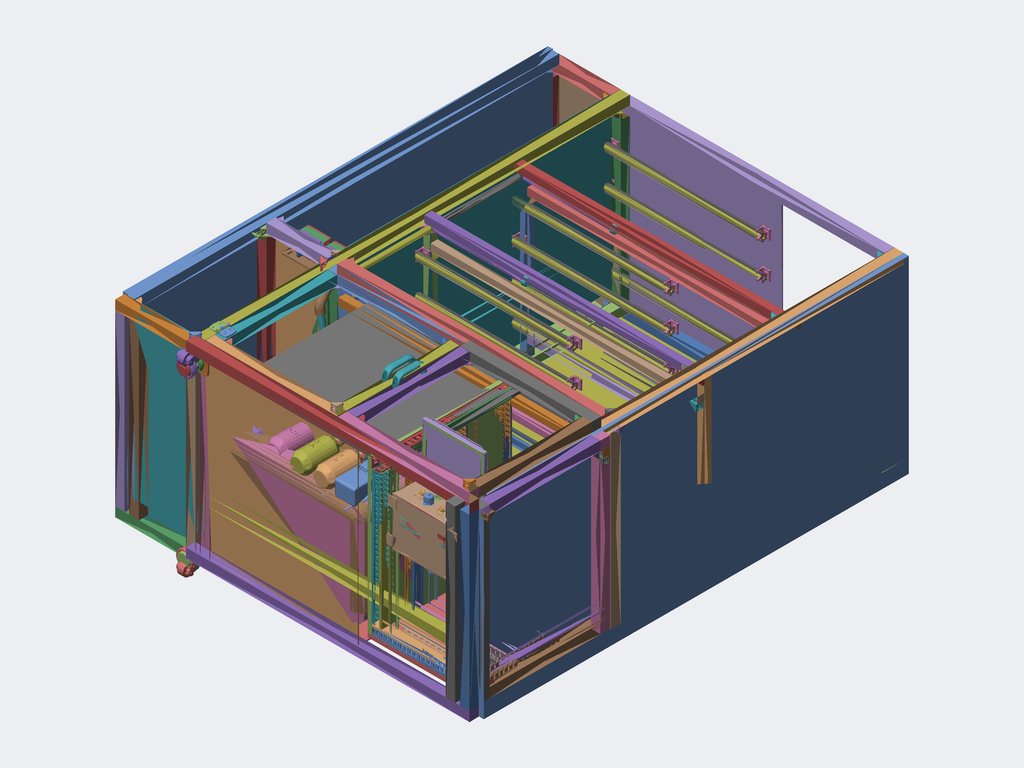Assembly | SolidWorks | 365 different items | 685 placed
Parts list (item | name | quantity | parent item | size | volume | features):
1 | (subassembly) | x1 | in 12 | 29 x 29.4 x 29.4 mm | 8063 mm3 | -
2 | (subassembly) | x1 | in 52 | 13.5 x 25.199 x 16.948 mm | 1807 mm3 | -
3 | (subassembly) | x1 | in 52 | 13.5 x 25.199 x 16.948 mm | 1807 mm3 | -
4 | (subassembly) | x1 | in 52 | 13.5 x 25.199 x 16.948 mm | 1807 mm3 | -
5 | (subassembly) | x1 | in 52 | 13.5 x 25.199 x 16.948 mm | 1807 mm3 | -
6 | (subassembly) | x1 | in 52 | - | - | -
7 | (subassembly) | x1 | in 52 | - | - | -
8 | (subassembly) | x1 | in 52 | - | - | -
9 | (subassembly) | x1 | in 52 | - | - | -
10 | (subassembly) | x1 | in 52 | - | - | -
11 | (subassembly) | x1 | in 52 | - | - | -
12 | (subassembly) | x1 | - | - | 806257 mm3 | -
13 | (subassembly) | x1 | in 50 | 13.5 x 25.199 x 16.948 mm | 1807 mm3 | -
14 | (subassembly) | x1 | in 124 | 23.449 x 13.5 x 13.5 mm | 1807 mm3 | -
15 | (subassembly) | x1 | in 53 | 13.5 x 26.207 x 19.88 mm | 1807 mm3 | -
16 | (subassembly) | x1 | in 53 | 13.5 x 26.207 x 19.88 mm | 1807 mm3 | -
17 | (subassembly) | x1 | in 53 | 13.5 x 26.207 x 19.88 mm | 1807 mm3 | -
18 | (subassembly) | x1 | in 53 | 13.5 x 26.207 x 19.88 mm | 1807 mm3 | -
19 | (subassembly) | x1 | in 53 | - | - | -
20 | (subassembly) | x1 | in 53 | - | - | -
21 | (subassembly) | x1 | in 53 | - | - | -
22 | (subassembly) | x1 | in 53 | - | - | -
23 | (subassembly) | x1 | in 80 | 664 x 385.75 x 394.5 mm | 131312 mm3 | -
24 | (subassembly) | x1 | in 53 | - | - | -
25 | (subassembly) | x1 | in 50 | - | - | -
26 | (subassembly) | x1 | in 53 | - | - | -
27 | (subassembly) | x1 | in 54 | 13.5 x 26.207 x 19.88 mm | 1807 mm3 | -
28 | (subassembly) | x1 | in 54 | 13.5 x 26.207 x 19.88 mm | 1807 mm3 | -
29 | (subassembly) | x1 | in 54 | 13.5 x 26.207 x 19.88 mm | 1807 mm3 | -
30 | (subassembly) | x1 | in 54 | 13.5 x 26.207 x 19.88 mm | 1807 mm3 | -
31 | (subassembly) | x1 | in 54 | - | - | -
32 | (subassembly) | x1 | in 54 | - | - | -
33 | (subassembly) | x1 | in 50 | - | - | -
34 | (subassembly) | x1 | - | 70 x 130 x 53 mm | 112751 mm3 | -
35 | (subassembly) | x1 | in 54 | - | - | -
36 | (subassembly) | x1 | in 55 | 13.5 x 26.207 x 19.88 mm | 1807 mm3 | -
37 | (subassembly) | x1 | in 55 | 13.5 x 26.207 x 19.88 mm | 1807 mm3 | -
38 | (subassembly) | x1 | in 55 | 13.5 x 26.207 x 19.88 mm | 1807 mm3 | -
39 | (subassembly) | x1 | in 55 | 13.5 x 26.207 x 19.88 mm | 1807 mm3 | -
40 | (subassembly) | x1 | in 55 | - | - | -
41 | (subassembly) | x1 | in 55 | - | - | -
42 | (subassembly) | x1 | in 55 | - | - | -
43 | (subassembly) | x1 | in 55 | - | - | -
44 | (subassembly) | x1 | in 55 | - | - | -
45 | (subassembly) | x1 | - | 77 x 48 x 16 mm | 26381 mm3 | -
46 | (subassembly) | x1 | in 50 | - | - | -
47 | (subassembly) | x1 | in 50 | - | - | -
48 | (subassembly) | x1 | in 50 | - | - | -
49 | (subassembly) | x1 | in 50 | - | - | -
50 | (subassembly) | x1 | in 126 | 346.5 x 25.199 x 16.948 mm | 7226 mm3 | -
51 | (subassembly) | x1 | in 127 | 346.5 x 25.199 x 16.948 mm | 7226 mm3 | -
52 | (subassembly) | x1 | in 129 | 346.5 x 25.199 x 16.948 mm | 7226 mm3 | -
53 | (subassembly) | x1 | in 113 | 346.5 x 26.207 x 19.88 mm | 7226 mm3 | -
54 | (subassembly) | x1 | in 114 | 346.5 x 26.207 x 19.88 mm | 7226 mm3 | -
55 | (subassembly) | x1 | in 115 | 346.5 x 26.207 x 19.88 mm | 7226 mm3 | -
56 | (subassembly) | x1 | in 45 | - | - | -
57 | (subassembly) | x1 | in 76 | 408 x 327.5 x 71.18 mm | 128215 mm3 | -
58 | (subassembly) | x1 | in 59 | 610 x 320 x 430 mm | 61319662 mm3 | -
59 | (subassembly) | x1 | - | - | - | -
60 | (subassembly) | x5 | in 97 | 23.094 x 55.999 x 32.35 mm | 8057 mm3 | -
61 | (subassembly) | x1 | in 98 | 23.094 x 55.999 x 32.35 mm | 8057 mm3 | -
62 | (subassembly) | x1 | in 99 | 23.094 x 55.999 x 32.35 mm | 8057 mm3 | -
63 | (subassembly) | x1 | in 137 | 41.648 x 27.781 x 48.022 mm | 12703 mm3 | -
64 | (subassembly) | x1 | in 137 | - | - | -
65 | (subassembly) | x1 | in 116 | 38.308 x 50.8 x 53.348 mm | 36744 mm3 | -
66 | (subassembly) | x5 | in 91 | 660 x 66.14 x 97.82 mm | 1407720 mm3 | -
67 | (subassembly) | x2 | in 45 | - | - | -
68 | (subassembly) | x1 | in 92 | 660 x 66.14 x 97.82 mm | 1407720 mm3 | -
69 | (subassembly) | x1 | in 93 | 660 x 66.14 x 97.82 mm | 1407720 mm3 | -
70 | (subassembly) | x1 | in 77 | 56.3 x 65.53 x 50.125 mm | 38385 mm3 | -
71 | (subassembly) | x1 | in 77 | 56.3 x 65.53 x 50.125 mm | 38385 mm3 | -
72 | (subassembly) | x1 | in 77 | 56.3 x 65.53 x 50.125 mm | 38385 mm3 | -
73 | (subassembly) | x1 | in 119 | - | - | -
74 | (subassembly) | x1 | in 77 | 56.3 x 65.53 x 50.125 mm | 38385 mm3 | -
75 | (subassembly) | x1 | in 77 | 56.3 x 65.53 x 50.125 mm | 38385 mm3 | -
76 | (subassembly) | x1 | in 59 | - | 1784290 mm3 | -
77 | (subassembly) | x1 | in 76 | - | 191920 mm3 | -
78 | (subassembly) | x1 | in 116 | 44.298 x 85.549 x 87.319 mm | 55176 mm3 | -
79 | (subassembly) | x1 | in 120 | 6.25 x 60 x 64.152 mm | 14252 mm3 | -
80 | (subassembly) | x1 | - | - | - | -
81 | (subassembly) | x1 | in 59 | 27.5 x 27.5 x 265.5 mm | 30904 mm3 | -
82 | (subassembly) | x1 | in 88 | - | - | -
83 | (subassembly) | x1 | in 88 | - | - | -
84 | (subassembly) | x3 | in 95, 106, 117 | 32.512 x 58.766 x 128.692 mm | 33883 mm3 | -
85 | (subassembly) | x1 | in 88 | 101 x 80 x 82.8 mm | 248675 mm3 | -
86 | (subassembly) | x1 | in 88 | - | - | -
87 | (subassembly) | x1 | in 88 | 101 x 80 x 82.8 mm | 248693 mm3 | -
88 | (subassembly) | x1 | - | 80 x 82.8 x 822 mm | 497420 mm3 | -
89 | (subassembly) | x1 | - | 676.368 x 834.5 x 490.186 mm | 2486985 mm3 | -
90 | (subassembly) | x3 | in 89 | 676.368 x 34.5 x 490.186 mm | 828995 mm3 | -
91 | (subassembly) | x5 | in 97 | 664 x 107.82 x 71.14 mm | 1474678 mm3 | -
92 | (subassembly) | x1 | in 98 | 664 x 107.82 x 71.14 mm | 1474678 mm3 | -
93 | (subassembly) | x1 | in 99 | 664 x 107.82 x 71.14 mm | 1474678 mm3 | -
94 | (subassembly) | x1 | - | - | 7857189 mm3 | -
95 | (subassembly) | x1 | in 126 | 174.317 x 60.383 x 32.544 mm | 89512 mm3 | -
96 | (subassembly) | x1 | in 94 | - | 7857189 mm3 | -
97 | (subassembly) | x5 | in 96, 100 | 107.82 x 101.739 x 678.552 mm | 1521216 mm3 | -
98 | (subassembly) | x1 | in 100 | 107.82 x 101.739 x 678.552 mm | 1521216 mm3 | -
99 | (subassembly) | x1 | in 100 | 107.82 x 101.739 x 678.552 mm | 1521216 mm3 | -
100 | (subassembly) | x1 | in 96 | - | 4563696 mm3 | -
101 | (subassembly) | x5 | in 97 | 17.4 x 36.23 x 48.652 mm | 7597 mm3 | -
102 | (subassembly) | x1 | in 98 | 17.4 x 36.23 x 48.652 mm | 7597 mm3 | -
103 | (subassembly) | x1 | in 99 | 17.4 x 36.23 x 48.652 mm | 7597 mm3 | -
104 | (subassembly) | x1 | in 125 | - | 2028858 mm3 | -
105 | (subassembly) | x1 | - | 1112 x 1800 x 795 mm | 20539975 mm3 | -
106 | (subassembly) | x1 | in 127 | 174.317 x 60.383 x 32.544 mm | 89512 mm3 | -
107 | (subassembly) | x1 | in 137 | 56.5 x 114.123 x 126.119 mm | 204524 mm3 | -
108 | (subassembly) | x1 | in 137 | 162.238 x 114.123 x 56.5 mm | 232338 mm3 | -
109 | (subassembly) | x5 | in 97 | 48.245 x 49.817 x 548.245 mm | 30830 mm3 | -
110 | (subassembly) | x1 | in 98 | 48.245 x 49.817 x 548.245 mm | 30830 mm3 | -
111 | (subassembly) | x1 | in 99 | 48.245 x 49.817 x 548.245 mm | 30830 mm3 | -
112 | (subassembly) | x1 | in 76 | - | 1269065 mm3 | -
113 | (subassembly) | x1 | in 116 | 422.844 x 53.25 x 32.766 mm | 119416 mm3 | -
114 | (subassembly) | x1 | in 116 | 426.966 x 53.25 x 32.766 mm | 119416 mm3 | -
115 | (subassembly) | x1 | in 116 | 422.797 x 53.25 x 32.766 mm | 119416 mm3 | -
116 | (subassembly) | x1 | in 125 | 428.236 x 959.541 x 415.929 mm | 725638 mm3 | -
117 | (subassembly) | x1 | in 129 | 174.317 x 60.383 x 32.544 mm | 89512 mm3 | -
118 | (subassembly) | x1 | in 120 | - | 494108 mm3 | -
119 | (subassembly) | x1 | - | - | - | -
120 | (subassembly) | x1 | in 73 | - | - | -
121 | (subassembly) | x1 | in 73 | 292.1 x 154.813 x 421.143 mm | 614239 mm3 | -
122 | (subassembly) | x1 | in 126 | 388.057 x 91.084 x 21.234 mm | 100985 mm3 | -
123 | (subassembly) | x2 | in 127, 129 | 388.057 x 91.084 x 21.234 mm | 100985 mm3 | -
124 | (subassembly) | x1 | in 104 | 38.38 x 1164 x 21.234 mm | 226503 mm3 | -
125 | (subassembly) | x1 | - | - | 2759072 mm3 | -
126 | (subassembly) | x1 | in 104 | 415.26 x 140.383 x 32.766 mm | 299661 mm3 | -
127 | (subassembly) | x1 | in 104 | 415.26 x 140.383 x 32.766 mm | 299661 mm3 | -
128 | (subassembly) | x1 | in 105 | 982 x 1800 x 795 mm | 20539975 mm3 | -
129 | (subassembly) | x1 | in 104 | 432.043 x 140.383 x 32.766 mm | 310066 mm3 | -
130 | (subassembly) | x5 | in 101 | 17.4 x 34.9 x 11.547 mm | 2470 mm3 | -
131 | (subassembly) | x1 | in 102 | 17.4 x 34.9 x 11.547 mm | 2470 mm3 | -
132 | (subassembly) | x1 | in 103 | 17.4 x 34.9 x 11.547 mm | 2470 mm3 | -
133 | (subassembly) | x1 | in 135 | 14 x 137.38 x 15.856 mm | 6154 mm3 | -
134 | (subassembly) | x1 | in 135 | 156 x 156 x 86 mm | 282738 mm3 | -
135 | (subassembly) | x1 | in 59 | 156 x 335.859 x 98.479 mm | 1667612 mm3 | -
136 | (subassembly) | x1 | in 108 | 79 x 109.5 x 56.5 mm | 176709 mm3 | -
137 | (subassembly) | x1 | in 104 | 415.889 x 172.793 x 383.815 mm | 846980 mm3 | features CompositeCurve 4
138 | (subassembly) | x1 | in 59 | 134.4 x 256.29 x 184.2 mm | 2229611 mm3 | -
139 | (subassembly) | x1 | in 12 | 29 x 29.4 x 29.4 mm | 8063 mm3 | -
140 | (subassembly) | x1 | in 137 | 69.85 x 87.046 x 27.178 mm | 35204 mm3 | -
141 | (subassembly) | x1 | in 137 | - | - | -
142 | (subassembly) | x1 | in 137 | 69.85 x 87.046 x 27.178 mm | 35204 mm3 | -
143 | (subassembly) | x1 | in 140 | 22.25 x 60.757 x 25.693 mm | 8431 mm3 | -
144 | (subassembly) | x1 | in 142 | 22.25 x 60.757 x 25.693 mm | 8431 mm3 | -
145 | (subassembly) | x1 | in 116 | 25.302 x 60.757 x 24.143 mm | 8431 mm3 | -
146 | (subassembly) | x1 | in 80 | - | - | -
147 | (subassembly) | x1 | in 50 | 13.5 x 25.199 x 16.948 mm | 1807 mm3 | -
148 | (subassembly) | x1 | in 50 | 13.5 x 25.199 x 16.948 mm | 1807 mm3 | -
149 | (subassembly) | x1 | in 51 | 13.5 x 25.199 x 16.948 mm | 1807 mm3 | -
150 | (subassembly) | x10 | in 12 | 29 x 29.4 x 29.4 mm | 8063 mm3 | -
151 | (subassembly) | x1 | in 51 | 13.5 x 25.199 x 16.948 mm | 1807 mm3 | -
152 | (subassembly) | x1 | in 51 | 13.5 x 25.199 x 16.948 mm | 1807 mm3 | -
153 | (subassembly) | x1 | in 51 | 13.5 x 25.199 x 16.948 mm | 1807 mm3 | -
154 | (subassembly) | x1 | in 51 | - | - | -
155 | (subassembly) | x1 | in 51 | - | - | -
156 | (subassembly) | x1 | in 51 | - | - | -
157 | (subassembly) | x1 | in 51 | - | - | -
158 | (subassembly) | x1 | in 51 | - | - | -
159 | (subassembly) | x1 | in 51 | - | - | -
160 | (subassembly) | x1 | in 50 | 13.5 x 25.199 x 16.948 mm | 1807 mm3 | -
161 | - | x1 | in 120 | 7.5 x 222.25 x 35 mm | 9598 mm3 | features BaseBody 1
162 | - | x1 | in 12 | 29 x 29.4 x 29.4 mm | 8063 mm3 | features BaseBody 1
163 | - | x1 | in 12 | 29 x 29.4 x 29.4 mm | 8063 mm3 | features BaseBody 1
164 | - | x1 | in 12 | 29 x 29.4 x 29.4 mm | 8063 mm3 | features BaseBody 1
165 | - | x1 | in 12 | 29 x 29.4 x 29.4 mm | 8063 mm3 | features BaseBody 1
166 | - | x1 | in 12 | 29 x 29.4 x 29.4 mm | 8063 mm3 | features BaseBody 1
167 | - | x1 | in 12 | 29 x 29.4 x 29.4 mm | 8063 mm3 | features BaseBody 1
168 | - | x1 | in 12 | 29 x 29.4 x 29.4 mm | 8063 mm3 | features BaseBody 1
169 | - | x1 | in 12 | 29 x 29.4 x 29.4 mm | 8063 mm3 | features BaseBody 1
170 | - | x1 | in 12 | 29 x 29.4 x 29.4 mm | 8063 mm3 | features BaseBody 1
171 | - | x1 | in 12 | 29 x 29.4 x 29.4 mm | 8063 mm3 | features BaseBody 1
172 | - | x4 | in 137, 143, 144, 145 | 22.25 x 25.693 x 60.757 mm | 8431 mm3 | features BaseBody 1
173 | - | x1 | in 12 | 29 x 29.4 x 29.4 mm | 8063 mm3 | features BaseBody 1
174 | - | x1 | in 12 | 29 x 29.4 x 29.4 mm | 8063 mm3 | features BaseBody 1
175 | - | x1 | in 12 | 29 x 29.4 x 29.4 mm | 8063 mm3 | features BaseBody 1
176 | - | x1 | in 12 | 29 x 29.4 x 29.4 mm | 8063 mm3 | features BaseBody 1
177 | - | x1 | in 12 | 29 x 29.4 x 29.4 mm | 8063 mm3 | features BaseBody 1
178 | - | x1 | in 12 | 29 x 29.4 x 29.4 mm | 8063 mm3 | features BaseBody 1
179 | - | x1 | in 12 | 29 x 29.4 x 29.4 mm | 8063 mm3 | features BaseBody 1
180 | - | x1 | in 12 | 29 x 29.4 x 29.4 mm | 8063 mm3 | features BaseBody 1
181 | - | x1 | in 12 | 29 x 29.4 x 29.4 mm | 8063 mm3 | features BaseBody 1
182 | - | x12 | in 1, 139, 150 | 29 x 29.4 x 29.4 mm | 8063 mm3 | features BaseBody 1
183 | - | x1 | in 112 | 85.56 x 83.56 x 203.378 mm | 49544 mm3 | features BaseBody 2
184 | - | x1 | in 135 | 67.479 x 24 x 282.859 mm | 49181 mm3 | features BaseBody 4
185 | - | x8 | in 104, 113, 114, 115, 126, 127, 129, 137 | 49.53 x 49.53 x 29.465 mm | 26737 mm3 | features BaseBody 1
186 | - | x1 | in 85 | 101 x 80 x 82.8 mm | 248675 mm3 | features BaseBody 9
187 | - | x1 | in 87 | 101 x 80 x 82.8 mm | 248693 mm3 | features BaseBody 9
188 | - | x12 | in 90 | 670 x 24 x 40.186 mm | 190097 mm3 | features BaseBody 2, ICE 1
189 | - | x1 | in 121 | 206.936 x 292.1 x 154.813 mm | 362955 mm3 | features BaseBody 1
190 | - | x1 | in 45 | 77 x 48 x 16 mm | 26381 mm3 | features BaseBody 3
191 | - | x1 | in 138 | 134.4 x 184.2 x 103.29 mm | 334800 mm3 | features BaseBody 3
192 | - | x7 | in 101, 102, 103 | - | 2700 mm3 | features BaseBody 1
193 | - | x2 | in 79, 120 | 64.028 x 5 x 60 mm | 11357 mm3 | features BaseBody 1
194 | - | x5 | in 70, 71, 72, 74, 75 | 65.53 x 40.25 x 56.3 mm | 27428 mm3 | features BaseBody 3
195 | - | x1 | in 79 | 63.246 x 1.25 x 48.204 mm | 2895 mm3 | features BaseBody 1
196 | - | x1 | in 120 | 43.7 x 5.75 x 42 mm | 7228 mm3 | features BaseBody 1
197 | - | x2 | - | 800 x 1800 x 20 mm | 28800000 mm3 | features Extrusion 1
198 | - | x1 | in 81 | 18.244 x 265.5 x 15.8 mm | 6663 mm3 | features BaseBody 1
199 | - | x1 | in 138 | 134.4 x 134.4 x 157.5 mm | 1797413 mm3 | features BaseBody 2
200 | - | x11 | in 95, 106, 107, 108, 117, 137 | 61.119 x 35.745 x 32.544 mm | 27815 mm3 | features BaseBody 2
201 | - | x1 | in 112 | 85.56 x 83.56 x 203.378 mm | 49595 mm3 | features BaseBody 2
202 | - | x1 | in 112 | 85.56 x 83.56 x 203.378 mm | 49646 mm3 | features BaseBody 2
203 | - | x1 | in 81 | - | - | features RefSurface 1
204 | - | x7 | in 60, 61, 62 | 23.094 x 24.5 x 20 mm | 3796 mm3 | features BaseBody 2
205 | - | x5 | in 70, 71, 72, 74, 75 | 19.6 x 11.9 x 19.6 mm | 729.046 mm3 | features BaseBody 1
206 | - | x1 | in 76 | 525 x 80 x 5 mm | 194805 mm3 | features BaseBody 11
207 | - | x1 | in 80 | 666 x 555 x 451 mm | 9776880 mm3 | features BaseBody 2
208 | - | x2 | in 73 | 50.41 x 34 x 34 mm | 20764 mm3 | features BaseBody 1
209 | - | x1 | in 73 | 26 x 30.7 x 31 mm | 6883 mm3 | features BaseBody 1
210 | - | x1 | in 124 | 21.234 x 384.346 x 21.234 mm | 76950 mm3 | features BaseBody 1
211 | - | x1 | in 124 | 21.234 x 384.6 x 21.234 mm | 78104 mm3 | features BaseBody 1
212 | - | x1 | in 124 | 21.234 x 344.346 x 21.234 mm | 69645 mm3 | features BaseBody 1
213 | - | x3 | in 113, 114, 115 | 381 x 21.235 x 21.234 mm | 75088 mm3 | features BaseBody 1, ICE 1
214 | - | x1 | in 116 | 86.694 x 862.008 x 383.174 mm | 199579 mm3 | features BaseBody 3
215 | - | x1 | in 133 | 14 x 15.856 x 22.23 mm | 2429 mm3 | features BaseBody 2
216 | - | x5 | in 70, 71, 72, 74, 75 | 39.14 x 10.37 x 38.9 mm | 2813 mm3 | features BaseBody 1
217 | - | x1 | in 133 | 14 x 15.856 x 22.23 mm | 1913 mm3 | features BaseBody 2
218 | - | x7 | in 101, 102, 103 | 14 x 15.856 x 22.23 mm | 2429 mm3 | features BaseBody 2
219 | - | x1 | - | 1190 x 1150 x 790 mm | 14724000 mm3 | features BaseBody 16
220 | - | x1 | - | 1500 x 1840 x 800 mm | 56736000 mm3 | features BaseBody 43
221 | - | x1 | in 138 | - | - | features BaseBody 2, RefSurface 1
222 | - | x1 | in 134 | 3 x 15 x 60 mm | 2677 mm3 | features BaseBody 1
223 | - | x1 | in 136 | 79 x 56.5 x 109.5 mm | 176709 mm3 | features BaseBody 10
224 | - | x2 | in 107, 137 | 79 x 56.5 x 109.5 mm | 176709 mm3 | features BaseBody 10
225 | - | x9 | in 116, 126, 127, 129, 137 | 70.104 x 49.555 x 29.007 mm | 32399 mm3 | features BaseBody 1
226 | - | x49 | in 109, 110, 111 | 48.245 x 48.245 x 49.817 mm | 4404 mm3 | features BaseBody 1
227 | - | x5 | in 70, 71, 72, 74, 75 | 31.23 x 17.45 x 36.34 mm | 4500 mm3 | features BaseBody 1
228 | - | x1 | - | 1160 x 720 x 3 mm | 2505600 mm3 | features Extrusion 1
229 | - | x1 | - | 720 x 260 x 5 mm | 936000 mm3 | features Extrusion 1
230 | - | x1 | in 146 | 40 x 40.1 x 555 mm | 152024 mm3 | features BaseBody 2
231 | - | x1 | in 146 | 40 x 40.1 x 555 mm | 152024 mm3 | features BaseBody 2
232 | - | x1 | in 146 | 40 x 40.1 x 395 mm | 108160 mm3 | features BaseBody 2
233 | - | x3 | in 146 | 40 x 40.1 x 395 mm | 108160 mm3 | features BaseBody 2
234 | - | x1 | in 146 | 40 x 40.1 x 570 mm | 156325 mm3 | features BaseBody 2
235 | - | x3 | in 146 | 40 x 40.1 x 570 mm | 156325 mm3 | features BaseBody 2
236 | - | x1 | in 58 | 608 x 220 x 428 mm | 56795852 mm3 | features BaseBody 1
237 | - | x1 | in 135 | 144 x 115 x 74 mm | 1223728 mm3 | features BaseBody 1
238 | - | x10 | in 70, 71, 72, 74, 75 | 7.18 x 1.7 x 7.64 mm | 58.331 mm3 | features BaseBody 1
239 | - | x1 | in 112 | 85 x 70 x 206 mm | 1070549 mm3 | features BaseBody 2
240 | - | x1 | in 96 | 355 x 5 x 135 mm | 128920 mm3 | features BaseBody 1, ICE 1
241 | - | x1 | in 134 | 150 x 153 x 80 mm | 237530 mm3 | features BaseBody 1
242 | - | x1 | in 23 | 7.5 x 35 x 637 mm | 27495 mm3 | features BaseBody 1
243 | - | x1 | in 23 | 7.5 x 35 x 386 mm | 16663 mm3 | features BaseBody 1
244 | - | x1 | in 23 | 7.5 x 35 x 386 mm | 16663 mm3 | features BaseBody 1
245 | - | x1 | in 23 | 7.5 x 35 x 386 mm | 16663 mm3 | features BaseBody 1
246 | - | x1 | in 23 | 7.5 x 35 x 637 mm | 27495 mm3 | features BaseBody 1
247 | - | x1 | in 23 | 7.5 x 35 x 610 mm | 26333 mm3 | features BaseBody 1
248 | - | x4 | in 81 | 16.932 x 14.78 x 0.889 mm | 89.694 mm3 | features BaseBody 1
249 | - | x15 | in 70, 71, 72, 74, 75 | 10.75 x 13.9 x 10.75 mm | 660.288 mm3 | features BaseBody 1
250 | - | x2 | in 81 | - | - | features RefSurface 1
251 | - | x2 | in 96 | 577 x 5 x 105 mm | 122030 mm3 | features BaseBody 1, ICE 1
252 | - | x1 | in 81 | 16 x 18.475 x 5 mm | 804.205 mm3 | features BaseBody 1
253 | - | x1 | in 134 | 156 x 8 x 86 mm | 42531 mm3 | features BaseBody 2
254 | - | x24 | in 90 | 40 x 32.5 x 32.5 mm | 8576 mm3 | features BaseBody 1
255 | - | x3 | in 122, 123 | 67 x 21.234 x 21.234 mm | 13325 mm3 | features BaseBody 1, ICE 1
256 | - | x1 | in 135 | 31.058 x 31.058 x 249.412 mm | 105798 mm3 | features BaseBody 5
257 | - | x9 | in 104, 113, 114, 115, 126, 127, 129 | 20.956 x 32.766 x 32.766 mm | 10405 mm3 | features BaseBody 1
258 | - | x7 | in 130, 131, 132 | 17.4 x 34.9 x 11.547 mm | 2470 mm3 | features BaseBody 4
259 | - | x3 | in 122, 123 | 290 x 21.234 x 21.234 mm | 58049 mm3 | features BaseBody 1
260 | - | x5 | in 70, 71, 72, 74, 75 | 21 x 4 x 40.5 mm | 817.162 mm3 | features BaseBody 1
261 | - | x7 | in 91, 92, 93 | 664 x 107.82 x 40 mm | 66958 mm3 | features BaseBody 2
262 | - | x7 | in 66, 68, 69 | 660 x 60.3 x 97.82 mm | 1057763 mm3 | features BaseBody 1
263 | - | x25 | in 2, 3, 4, 5, 13, 14, 15, 16, 17, 18, 27, 28, 29, 30, 36, 37, 38, 39, 147, 148, 149, 151, 152, 153, 160 | 13.5 x 13.5 x 23.449 mm | 1807 mm3 | features BaseBody 1
264 | - | x7 | in 66, 68, 69 | 660 x 11.68 x 97.82 mm | 349958 mm3 | features BaseBody 1
265 | - | x1 | in 133 | 6.9 x 97.77 x 6.9 mm | 1812 mm3 | features BaseBody 1
266 | - | x3 | in 122, 123 | 145.797 x 21.234 x 21.234 mm | 29608 mm3 | features BaseBody 1
267 | - | x1 | in 128 | 260 x 560 x 5 mm | 728000 mm3 | features BaseBody 1
268 | - | x1 | in 128 | 260 x 5 x 720 mm | 936000 mm3 | features BaseBody 1
269 | - | x1 | in 128 | 645 x 555 x 10 mm | 3579750 mm3 | features BaseBody 1, ICE 1
270 | - | x1 | in 128 | 647 x 1160 x 5 mm | 3752600 mm3 | features BaseBody 1, ICE 1
271 | - | x1 | in 120 | 25.3 x 89.537 x 86.5 mm | 117361 mm3 | features BaseBody 1
272 | - | x2 | in 34 | 130 x 53 x 26 mm | 56376 mm3 | features BaseBody 1
273 | - | x1 | in 128 | 330 x 5 x 790 mm | 1246600 mm3 | features BaseBody 1
274 | - | x1 | in 128 | 647 x 5 x 755 mm | 2438375 mm3 | features BaseBody 1, ICE 1
275 | - | x1 | in 128 | 647 x 5 x 685 mm | 2209850 mm3 | features BaseBody 1, ICE 1
276 | - | x1 | in 128 | 260 x 1160 x 5 mm | 1508000 mm3 | features BaseBody 1
277 | - | x1 | in 128 | 647 x 560 x 5 mm | 1811600 mm3 | features BaseBody 1, ICE 1
278 | - | x1 | in 128 | 647 x 5 x 720 mm | 2329200 mm3 | features BaseBody 1, ICE 1
279 | - | x7 | in 60, 61, 62 | 14.797 x 28.95 x 37.899 mm | 4262 mm3 | features BaseBody 4
280 | - | x1 | in 112 | 85.56 x 83.56 x 203.378 mm | 49716 mm3 | features BaseBody 2
281 | - | x1 | in 58 | 610 x 320 x 430 mm | 4523810 mm3 | features BaseBody 1
282 | - | x3 | in 73 | 28.575 x 26.721 x 28.575 mm | 6118 mm3 | features BaseBody 1
283 | - | x1 | in 118 | - | 331600 mm3 | features BaseBody 1
284 | - | x1 | in 118 | - | 162507 mm3 | features BaseBody 1
285 | - | x1 | in 121 | 174.625 x 222.25 x 1.829 mm | 70680 mm3 | features BaseBody 1
286 | - | x1 | in 121 | 216.967 x 261.925 x 18.699 mm | 126751 mm3 | features BaseBody 1
287 | - | x1 | in 121 | 204.775 x 6.35 x 255.575 mm | 53856 mm3 | features BaseBody 1
288 | - | x1 | in 120 | 130 x 37 x 131 mm | 590430 mm3 | features BaseBody 1
289 | - | x5 | in 57 | 8 x 327.5 x 71.18 mm | 25643 mm3 | features BaseBody 2
290 | - | x1 | in 12 | 29 x 29.4 x 29.4 mm | 8063 mm3 | features BaseBody 1
291 | - | x1 | in 12 | 29 x 29.4 x 29.4 mm | 8063 mm3 | features BaseBody 1
292 | - | x1 | in 12 | 29 x 29.4 x 29.4 mm | 8063 mm3 | features BaseBody 1
293 | - | x1 | in 12 | 29 x 29.4 x 29.4 mm | 8063 mm3 | features BaseBody 1
294 | - | x1 | in 12 | 29 x 29.4 x 29.4 mm | 8063 mm3 | features BaseBody 1
295 | - | x1 | in 12 | 29 x 29.4 x 29.4 mm | 8063 mm3 | features BaseBody 1
296 | - | x1 | in 12 | 29 x 29.4 x 29.4 mm | 8063 mm3 | features BaseBody 1
297 | - | x1 | in 12 | 29 x 29.4 x 29.4 mm | 8063 mm3 | features BaseBody 1
298 | - | x1 | in 12 | 29 x 29.4 x 29.4 mm | 8063 mm3 | features BaseBody 1
299 | - | x1 | in 65 | 51.054 x 50.8 x 32.512 mm | 36744 mm3 | features BaseBody 1
300 | - | x1 | in 12 | 29 x 29.4 x 29.4 mm | 8063 mm3 | features BaseBody 1
301 | - | x1 | in 12 | 29 x 29.4 x 29.4 mm | 8063 mm3 | features BaseBody 1
302 | - | x1 | in 12 | 29 x 29.4 x 29.4 mm | 8063 mm3 | features BaseBody 1
303 | - | x1 | in 12 | 29 x 29.4 x 29.4 mm | 8063 mm3 | features BaseBody 1
304 | - | x1 | in 12 | 29 x 29.4 x 29.4 mm | 8063 mm3 | features BaseBody 1
305 | - | x1 | in 12 | 29 x 29.4 x 29.4 mm | 8063 mm3 | features BaseBody 1
306 | - | x1 | in 12 | 29 x 29.4 x 29.4 mm | 8063 mm3 | features BaseBody 1
307 | - | x1 | in 12 | 29 x 29.4 x 29.4 mm | 8063 mm3 | features BaseBody 1
308 | - | x1 | in 12 | 29 x 29.4 x 29.4 mm | 8063 mm3 | features BaseBody 1
309 | - | x1 | in 12 | 29 x 29.4 x 29.4 mm | 8063 mm3 | features BaseBody 1
310 | - | x3 | in 137, 140, 142 | 69.85 x 48.514 x 27.178 mm | 26765 mm3 | features BaseBody 1
311 | - | x1 | in 12 | 29 x 29.4 x 29.4 mm | 8063 mm3 | features BaseBody 1
312 | - | x1 | in 12 | 29 x 29.4 x 29.4 mm | 8063 mm3 | features BaseBody 1
313 | - | x1 | in 12 | 29 x 29.4 x 29.4 mm | 8063 mm3 | features BaseBody 1
314 | - | x1 | in 12 | 29 x 29.4 x 29.4 mm | 8063 mm3 | features BaseBody 1
315 | - | x1 | in 12 | 29 x 29.4 x 29.4 mm | 8063 mm3 | features BaseBody 1
316 | - | x1 | in 12 | 29 x 29.4 x 29.4 mm | 8063 mm3 | features BaseBody 1
317 | - | x1 | in 12 | 29 x 29.4 x 29.4 mm | 8063 mm3 | features BaseBody 1
318 | - | x1 | in 12 | 29 x 29.4 x 29.4 mm | 8063 mm3 | features BaseBody 1
319 | - | x1 | in 12 | 29 x 29.4 x 29.4 mm | 8063 mm3 | features BaseBody 1
320 | - | x1 | in 12 | 29 x 29.4 x 29.4 mm | 8063 mm3 | features BaseBody 1
321 | - | x3 | in 84 | 32.512 x 58.766 x 128.692 mm | 33883 mm3 | features BaseBody 4
322 | - | x1 | in 12 | 29 x 29.4 x 29.4 mm | 8063 mm3 | features BaseBody 1
323 | - | x1 | in 12 | 29 x 29.4 x 29.4 mm | 8063 mm3 | features BaseBody 1
324 | - | x1 | in 12 | 29 x 29.4 x 29.4 mm | 8063 mm3 | features BaseBody 1
325 | - | x1 | in 12 | 29 x 29.4 x 29.4 mm | 8063 mm3 | features BaseBody 1
326 | - | x1 | in 12 | 29 x 29.4 x 29.4 mm | 8063 mm3 | features BaseBody 1
327 | - | x1 | in 12 | 29 x 29.4 x 29.4 mm | 8063 mm3 | features BaseBody 1
328 | - | x1 | in 12 | 29 x 29.4 x 29.4 mm | 8063 mm3 | features BaseBody 1
329 | - | x1 | in 12 | 29 x 29.4 x 29.4 mm | 8063 mm3 | features BaseBody 1
330 | - | x1 | in 12 | 29 x 29.4 x 29.4 mm | 8063 mm3 | features BaseBody 1
331 | - | x1 | in 12 | 29 x 29.4 x 29.4 mm | 8063 mm3 | features BaseBody 1
332 | - | x1 | in 63 | 27.781 x 48.022 x 41.648 mm | 12703 mm3 | features BaseBody 1
333 | - | x1 | in 12 | 29 x 29.4 x 29.4 mm | 8063 mm3 | features BaseBody 1
334 | - | x1 | in 12 | 29 x 29.4 x 29.4 mm | 8063 mm3 | features BaseBody 1
335 | - | x1 | in 12 | 29 x 29.4 x 29.4 mm | 8063 mm3 | features BaseBody 1
336 | - | x1 | in 12 | 29 x 29.4 x 29.4 mm | 8063 mm3 | features BaseBody 1
337 | - | x1 | in 12 | 29 x 29.4 x 29.4 mm | 8063 mm3 | features BaseBody 1
338 | - | x1 | in 12 | 29 x 29.4 x 29.4 mm | 8063 mm3 | features BaseBody 1
339 | - | x1 | in 12 | 29 x 29.4 x 29.4 mm | 8063 mm3 | features BaseBody 1
340 | - | x1 | in 12 | 29 x 29.4 x 29.4 mm | 8063 mm3 | features BaseBody 1
341 | - | x1 | in 12 | 29 x 29.4 x 29.4 mm | 8063 mm3 | features BaseBody 1
342 | - | x1 | in 12 | 29 x 29.4 x 29.4 mm | 8063 mm3 | features BaseBody 1
343 | - | x2 | in 78 | 48.046 x 60.492 x 32.512 mm | 27507 mm3 | features BaseBody 1
344 | - | x1 | in 12 | 29 x 29.4 x 29.4 mm | 8063 mm3 | features BaseBody 1
345 | - | x1 | in 12 | 29 x 29.4 x 29.4 mm | 8063 mm3 | features BaseBody 1
346 | - | x1 | in 12 | 29 x 29.4 x 29.4 mm | 8063 mm3 | features BaseBody 1
347 | - | x1 | in 12 | 29 x 29.4 x 29.4 mm | 8063 mm3 | features BaseBody 1
348 | - | x1 | in 12 | 29 x 29.4 x 29.4 mm | 8063 mm3 | features BaseBody 1
349 | - | x1 | in 12 | 29 x 29.4 x 29.4 mm | 8063 mm3 | features BaseBody 1
350 | - | x1 | in 12 | 29 x 29.4 x 29.4 mm | 8063 mm3 | features BaseBody 1
351 | - | x1 | in 12 | 29 x 29.4 x 29.4 mm | 8063 mm3 | features BaseBody 1
352 | - | x1 | in 12 | 29 x 29.4 x 29.4 mm | 8063 mm3 | features BaseBody 1
353 | - | x1 | in 12 | 29 x 29.4 x 29.4 mm | 8063 mm3 | features BaseBody 1
354 | - | x1 | in 120 | 80 x 37.1 x 92.55 mm | 180588 mm3 | features BaseBody 1
355 | - | x1 | in 12 | 29 x 29.4 x 29.4 mm | 8063 mm3 | features BaseBody 1
356 | - | x1 | in 12 | 29 x 29.4 x 29.4 mm | 8063 mm3 | features BaseBody 1
357 | - | x1 | in 12 | 29 x 29.4 x 29.4 mm | 8063 mm3 | features BaseBody 1
358 | - | x1 | in 12 | 29 x 29.4 x 29.4 mm | 8063 mm3 | features BaseBody 1
359 | - | x1 | in 12 | 29 x 29.4 x 29.4 mm | 8063 mm3 | features BaseBody 1
360 | - | x1 | in 12 | 29 x 29.4 x 29.4 mm | 8063 mm3 | features BaseBody 1
361 | - | x1 | in 12 | 29 x 29.4 x 29.4 mm | 8063 mm3 | features BaseBody 1
362 | - | x1 | in 12 | 29 x 29.4 x 29.4 mm | 8063 mm3 | features BaseBody 1
363 | - | x1 | in 12 | 29 x 29.4 x 29.4 mm | 8063 mm3 | features BaseBody 1
364 | - | x1 | in 12 | 29 x 29.4 x 29.4 mm | 8063 mm3 | features BaseBody 1
365 | - | x1 | in 120 | 17.6 x 73.879 x 84.3 mm | 78894 mm3 | features BaseBody 1
Mates (type | each side: item.copy, entity, surface, feature):
In the top assembly
Coincident | 220.1 face plane 输入12 | 197.1 face plane Boss-Extrude 1
Coincident | 220.1 face plane 输入22 | 229.1 face plane Boss-Extrude 1 | 2 times
Coincident | 220.1 face plane 输入11 | 228.1 face plane Boss-Extrude 1
Coincident | 220.1 face plane 输入21 | 228.1 face plane Boss-Extrude 1
Tangent | 261.1 face cylinder 输入1 | 251.1 face plane 输入1
Coincident | 229.1 face plane Boss-Extrude 1 | 251.1 face plane 输入1
Coincident | 262.1 face plane 输入1 | 262.2 face plane 输入1
Coincident | 262.1 face plane 输入1 | 262.3 face plane 输入1
Coincident | 262.2 face plane 输入1 | 251.1 face plane 输入1
Coincident | 220.1 face plane 输入31 | 197.2 face plane Boss-Extrude 1
Coincident | 220.1 face plane 输入13 | 197.2 face plane Boss-Extrude 1
Coincident | 220.1 face plane 输入36 | 197.2 face plane Boss-Extrude 1
In subassembly 137
Concentric | 224.1 edge | 310.1 edge
Coincident | 224.1 face plane 输入3 | 310.1 face plane 输入1
Concentric | 310.1 edge | 172.1 edge
Coincident | 310.1 face plane 输入1 | 172.1 face plane 输入1
In subassembly 128
Coordinate | 267.1 select_type:25 | 128.1 select_type:11
Coordinate | 270.1 select_type:25 | 128.1 select_type:11
Coordinate | 273.1 select_type:25 | 128.1 select_type:11
Coordinate | 274.1 select_type:25 | 128.1 select_type:11
Coordinate | 275.1 select_type:25 | 128.1 select_type:11
Coordinate | 276.1 select_type:25 | 128.1 select_type:11
Coordinate | 277.1 select_type:25 | 128.1 select_type:11
Coordinate | 278.1 select_type:25 | 128.1 select_type:11
Coordinate | 268.1 select_type:25 | 128.1 select_type:11